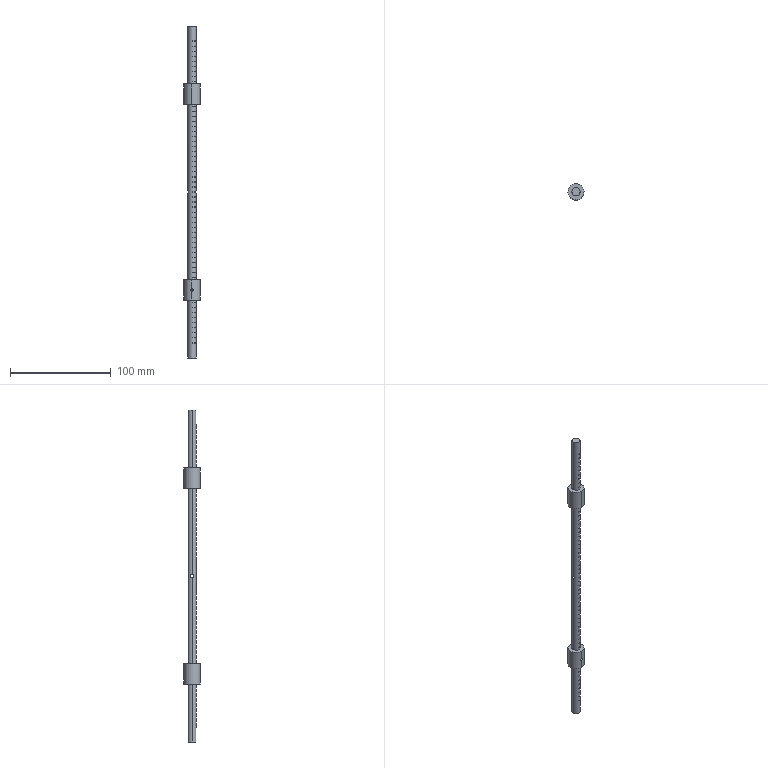Part | SolidWorks | features MirrorCompFeat 1, ReferencePattern 1 | 3 solids | 326 faces | box 16 x 16 x 330 mm | volume 22461 mm3 | plane 249 | cylinder 77 | commonest cylinder face diameters 7.8 x61 2.5 x4 8.1 x4 16 x4 3.2 x2 8 x2